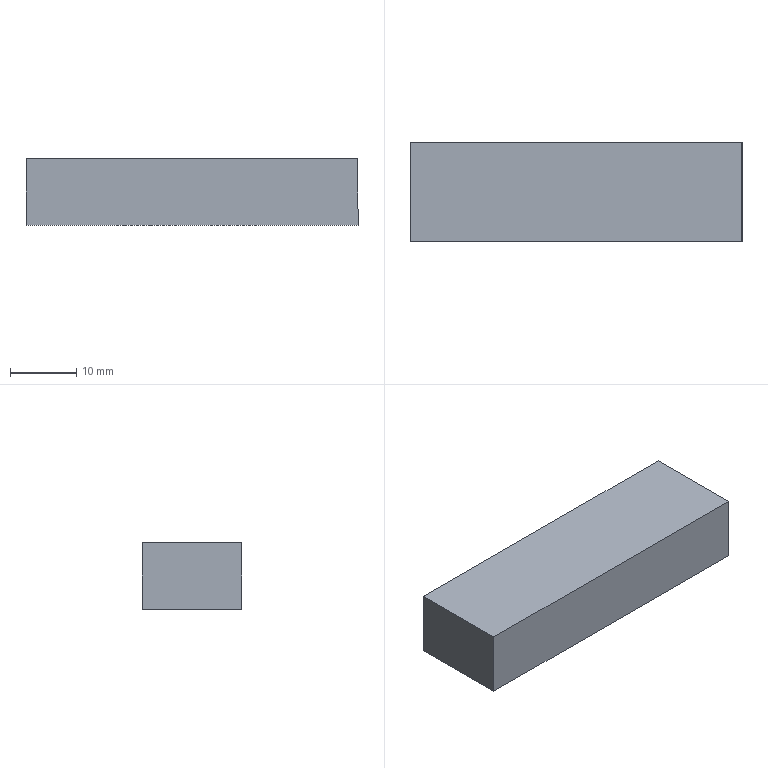CAM job | NX | 3+2 milling, drilling | part box 50 x 15 x 10 mm | stock box 50 x 15 x 10 mm
Tools:
number,name,description,diameter,corner_radius,flute_length,length,flutes
0,D2-7-D2-50-3T,D2-7-D2-50-3T,2.0,0.0,7.0,50.0,2
1,D8-25-D8-60-3T-ROUGH,D8-25-D8-60-3T-粗,8.0,0.0,25.0,60.0,2
2,D8-25-D8-60-3T-FINISH,D8-25-D8-60-3T,8.0,0.0,25.0,60.0,3
4,DRILLD2.3-29-55,钻刀D2.1-29-55,2.3,0.0,29.0,55.0,2
0,DRILLD2.5-35-61,钻刀D2.5-35-61,2.5,0.0,36.0,61.0,2
5,FORMTAPM2.5-12-D3-39,挤压M2.5-12-D3-39,2.5,0.0,13.0,15.0,2
0,TOPROWM3-10-D4-52,上排M3-10-D4-52,3.0,0.0,10.0,12.0,2
3,CHAMFERD4-90DEG,倒角D4-90度,4.0,0.0,5.0,50.0,2
0,CHAMFERD10-90DEG,倒角D10-90度,10.0,0.0,10.0,75.0,2
0,BALLNOSER1.5-6-D4-50,球刀R1.5-6-D4-50,3.0,1.5,6.0,6.5,2
Operations:
program,operation,operation_type,tool,method,geometry_group,spindle_rpm,surface_speed,feed_per_tooth,feed_cut,feed_plunge,cut_length_mm,path_length_mm,cut_time_min,machine_time_min
A1,DYNAMICROUGH,CavityMilling,D8-25-D8-60-3T-ROUGH,METHOD,WORKPIECE_54,6500.0,100.0,0.1178,3000.0,100.0,944.485,1665.51,0.3047,0.3768
A1,PLANAR_MILL_1,PlanarMilling,D8-25-D8-60-3T-FINISH,METHOD,WORKPIECE_54,4500.0,113.0,0.0593,800.0,100.0,37.6,153.6,0.047,0.0586
A1,PLANAR_MILL,PlanarMilling,D8-25-D8-60-3T-FINISH,METHOD,WORKPIECE_54,4500.0,113.0,0.0593,800.0,100.0,253.446,384.668,0.3168,0.3299
A1,FLOOR_WALL,VolumeBased25DMillingOperation,D8-25-D8-60-3T-FINISH,METHOD,WORKPIECE_54,4500.0,84.0,0.0889,800.0,100.0,94.797,142.797,0.1185,0.1233
A1,DRILLING,Operation,CHAMFERD4-90DEG,METHOD,WORKPIECE_54,3000.0,37.0,0.0333,200.0,0.0,8.6,99.129,0.043,0.0521
A1,PLANAR_MILL_3,PlanarMilling,CHAMFERD4-90DEG,METHOD,WORKPIECE_54,4000.0,50.0,0.125,1000.0,100.0,28.0,142.8,0.028,0.0395
A1,PLANAR_MILL_4,PlanarMilling,CHAMFERD4-90DEG,METHOD,WORKPIECE_54,4000.0,50.0,0.125,1000.0,100.0,55.59,168.391,0.0556,0.0669
A1,PLANAR_MILL_4_COPY,PlanarMilling,CHAMFERD4-90DEG,METHOD,WORKPIECE_54,4000.0,50.0,0.125,1000.0,100.0,65.883,181.883,0.0659,0.0775
A1,DRILLING_1,Operation,DRILLD2.3-29-55,METHOD,WORKPIECE_54,3000.0,21.0,0.0333,200.0,0.0,18.0,117.929,0.09,0.1
A1,DRILLING_1_COPY_1,Operation,D2-7-D2-50-3T,METHOD,WORKPIECE_54,3000.0,21.0,0.0333,200.0,0.0,18.0,117.929,0.09,0.1
A1,DRILLING_1_COPY,Operation,FORMTAPM2.5-12-D3-39,METHOD,WORKPIECE_54,300.0,2.0,0.0008,0.45,0.0,17.6,117.129,39.111,39.121
A1,PLANAR_MILL_2,PlanarMilling,BALLNOSER1.5-6-D4-50,METHOD,WORKPIECE_54,4500.0,84.0,0.0889,800.0,100.0,32.0,159.453,0.04,0.0527
B1,DRILLING_2,Operation,CHAMFERD4-90DEG,METHOD,B-G55,3000.0,37.0,0.0333,200.0,0.0,4.5,15.0,0.0225,0.0235
B1,DRILLING_2_COPY,Operation,DRILLD2.5-35-61,METHOD,B-G55,3000.0,37.0,0.0333,200.0,0.0,11.0,28.0,0.055,0.0567
B1,DRILLING_2_COPY_COPY,Operation,TOPROWM3-10-D4-52,METHOD,B-G55,300.0,2.0,0.0008,0.5,0.0,10.0,26.0,20.0,20.002
C1,PLANAR_MILL_5,PlanarMilling,D8-25-D8-60-3T-ROUGH,METHOD,C-G56,4500.0,113.0,0.1333,1200.0,100.0,300.0,632.25,0.25,0.2832
C1,ZLEVEL_PROFILE_STEEP,ZLevelMilling,D8-25-D8-60-3T-ROUGH,METHOD,C-G56,4500.0,113.0,0.2222,2000.0,100.0,47.8,201.743,0.0239,0.0393
C1,PLANAR_MILL_5_COPY,PlanarMilling,D8-25-D8-60-3T-FINISH,METHOD,C-G56,4500.0,113.0,0.0889,800.0,100.0,75.0,109.0,0.0937,0.0971
C1,PLANAR_MILL_6,PlanarMilling,CHAMFERD10-90DEG,METHOD,C-G56,3000.0,113.0,0.05,300.0,100.0,21.8,66.8,0.0727,0.0772
C1,PLANAR_MILL_7,PlanarMilling,CHAMFERD10-90DEG,METHOD,C-G56,4500.0,169.0,0.1111,1000.0,100.0,96.712,133.712,0.0967,0.1004